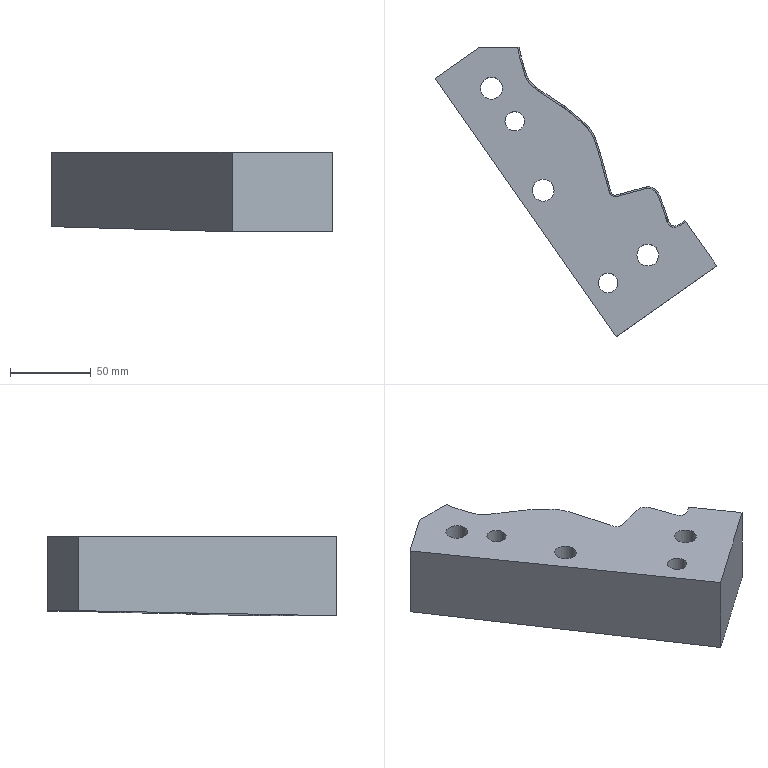Part | NX | features solid 2 | 1 solid | 25 faces | box 174.157 x 178.927 x 49.162 mm | volume 505819 mm3 | plane 13 | cylinder 10 | spline 2 | commonest cylinder face diameters 13.5 x3 19.5 x3 12 x2 13 x2